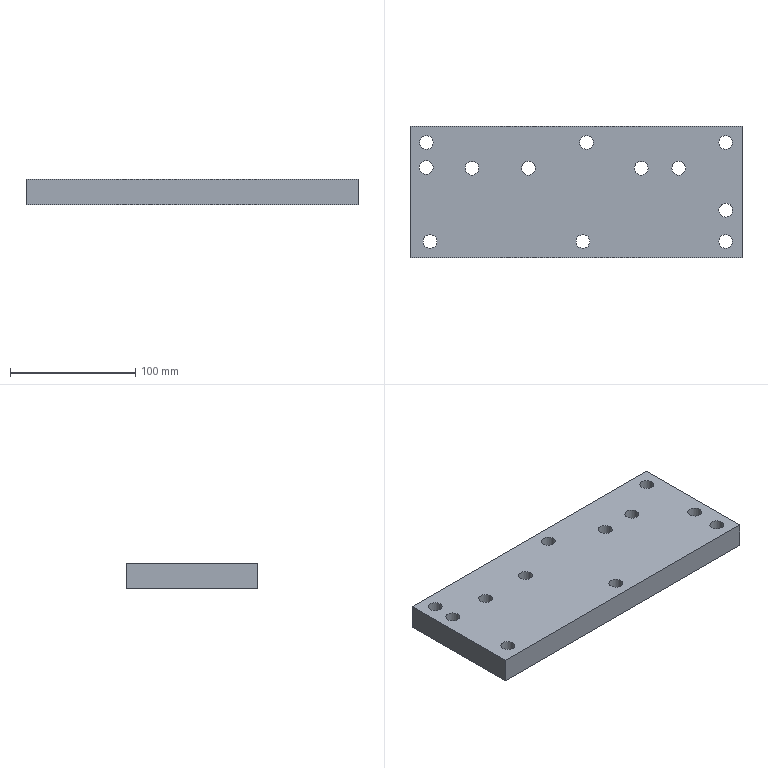Part | STEP file | 105_id3182_x_t | 1 solid | 18 faces | box 265 x 105 x 20 mm | volume 533692 mm3 | cylinder 12 | plane 6 | commonest cylinder face diameters 11 x12